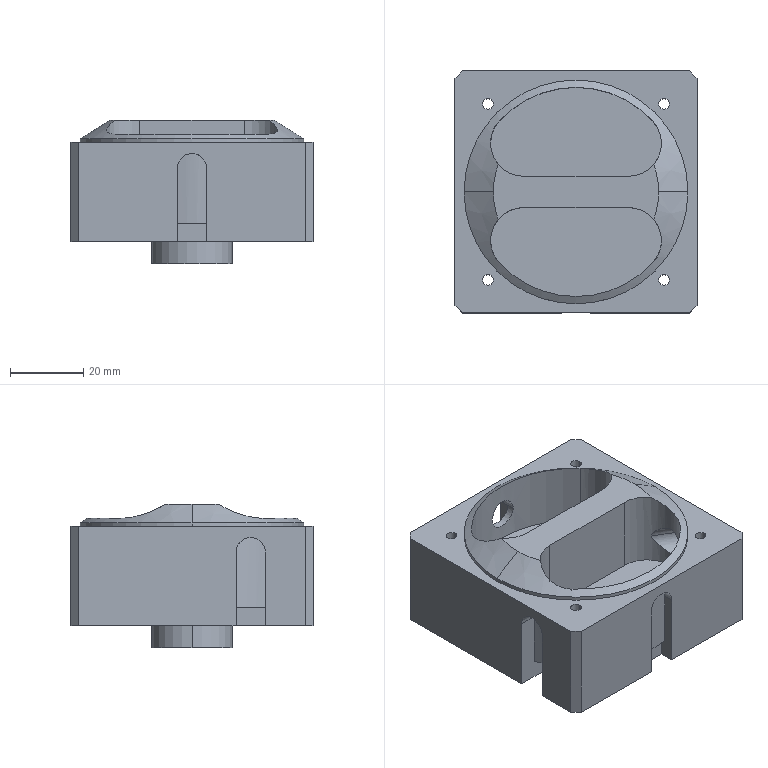Part | STEP file | ASND-0110-E63-HLTP01power supply C863_PI1#E5830 | 1 solid | 71 faces | box 66 x 66 x 39 mm | volume 89976 mm3 | plane 37 | cylinder 32 | cone 2 | commonest cylinder face diameters 2.932 x8 8 x7 61 x7 18 x6 22 x2 57 x2